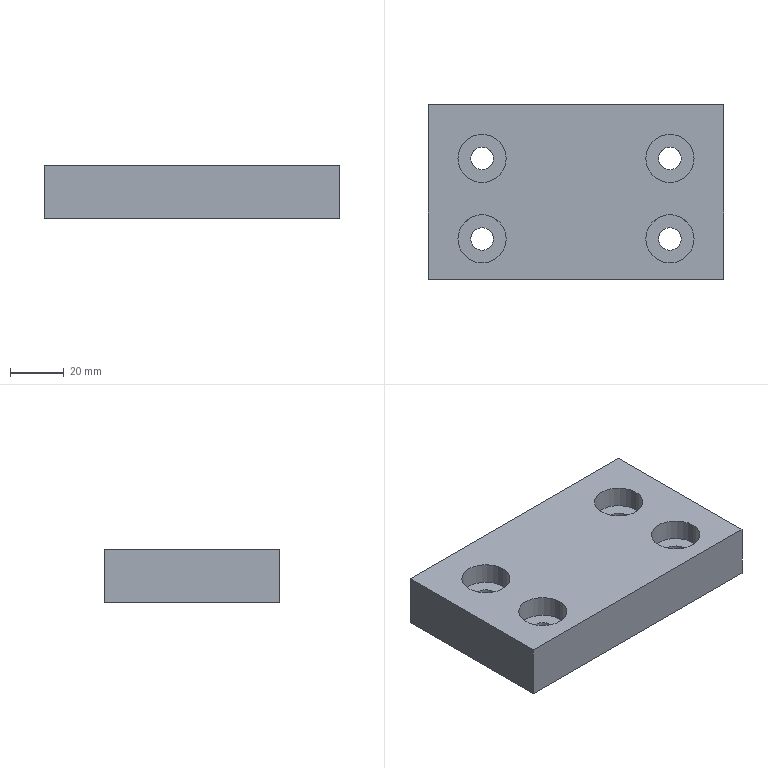Part | SolidWorks | features BaseBody 1 | 1 solid | 34 faces | box 110 x 65 x 20 mm | volume 129905 mm3 | cylinder 20 | plane 10 | cone 4 | commonest cylinder face diameters 8.4 x8 18 x8 10.2 x4
STEP:
#1=CARTESIAN_POINT('',(-264.2,110.,-32.879));
#2=VERTEX_POINT('',#1);
#3=CARTESIAN_POINT('',(-255.8,110.,-32.879));
#4=VERTEX_POINT('',#3);
#5=CARTESIAN_POINT('',(-260.,110.,-32.879));
#6=DIRECTION('',(0.,0.,1.));
#7=DIRECTION('',(1.,0.,0.));
#8=AXIS2_PLACEMENT_3D('',#5,#6,#7);
#9=CIRCLE('',#8,4.2);
#10=EDGE_CURVE('',#2,#4,#9,.T.);
#11=ORIENTED_EDGE('',*,*,#10,.F.);
#12=CARTESIAN_POINT('',(-264.2,110.,-20.879));
#13=VERTEX_POINT('',#12);
#14=CARTESIAN_POINT('',(-264.2,110.,-12.879));
#15=DIRECTION('',(0.,0.,1.));
#16=VECTOR('',#15,1000.);
#17=LINE('',#14,#16);
#18=EDGE_CURVE('',#2,#13,#17,.T.);
#19=ORIENTED_EDGE('',*,*,#18,.T.);
#20=CARTESIAN_POINT('',(-255.8,110.,-20.879));
#21=VERTEX_POINT('',#20);
#22=CARTESIAN_POINT('',(-260.,110.,-20.879));
#23=DIRECTION('',(0.,0.,-1.));
#24=DIRECTION('',(1.,0.,0.));
#25=AXIS2_PLACEMENT_3D('',#22,#23,#24);
#26=CIRCLE('',#25,4.2);
#27=EDGE_CURVE('',#21,#13,#26,.T.);
#28=ORIENTED_EDGE('',*,*,#27,.F.);
#29=CARTESIAN_POINT('',(-255.8,110.,-12.879));
#30=DIRECTION('',(0.,0.,1.));
#31=VECTOR('',#30,1000.);
#32=LINE('',#29,#31);
#33=EDGE_CURVE('',#4,#21,#32,.T.);
#34=ORIENTED_EDGE('',*,*,#33,.F.);
#35=EDGE_LOOP('',(#11,#19,#28,#34));
#36=FACE_OUTER_BOUND('',#35,.T.);
#37=CARTESIAN_POINT('',(-260.,110.,-12.879));
#38=DIRECTION('',(0.,0.,1.));
#39=DIRECTION('',(1.,0.,0.));
#40=AXIS2_PLACEMENT_3D('',#37,#38,#39);
#41=CYLINDRICAL_SURFACE('',#40,4.2);
#42=ADVANCED_FACE('',(#36),#41,.F.);
#43=CARTESIAN_POINT('',(-264.2,80.,-32.879));
#44=VERTEX_POINT('',#43);
#45=CARTESIAN_POINT('',(-255.8,80.,-32.879));
#46=VERTEX_POINT('',#45);
#47=CARTESIAN_POINT('',(-260.,80.,-32.879));
#48=DIRECTION('',(0.,0.,1.));
#49=DIRECTION('',(1.,0.,0.));
#50=AXIS2_PLACEMENT_3D('',#47,#48,#49);
#51=CIRCLE('',#50,4.2);
#52=EDGE_CURVE('',#44,#46,#51,.T.);
#53=ORIENTED_EDGE('',*,*,#52,.F.);
#54=CARTESIAN_POINT('',(-264.2,80.,-20.879));
#55=VERTEX_POINT('',#54);
#56=CARTESIAN_POINT('',(-264.2,80.,-12.879));
#57=DIRECTION('',(0.,0.,1.));
#58=VECTOR('',#57,1000.);
#59=LINE('',#56,#58);
#60=EDGE_CURVE('',#44,#55,#59,.T.);
#61=ORIENTED_EDGE('',*,*,#60,.T.);
#62=CARTESIAN_POINT('',(-255.8,80.,-20.879));
#63=VERTEX_POINT('',#62);
#64=CARTESIAN_POINT('',(-260.,80.,-20.879));
#65=DIRECTION('',(0.,0.,-1.));
#66=DIRECTION('',(1.,0.,0.));
#67=AXIS2_PLACEMENT_3D('',#64,#65,#66);
#68=CIRCLE('',#67,4.2);
#69=EDGE_CURVE('',#63,#55,#68,.T.);
#70=ORIENTED_EDGE('',*,*,#69,.F.);
#71=CARTESIAN_POINT('',(-255.8,80.,-12.879));
#72=DIRECTION('',(0.,0.,1.));
#73=VECTOR('',#72,1000.);
#74=LINE('',#71,#73);
#75=EDGE_CURVE('',#46,#63,#74,.T.);
#76=ORIENTED_EDGE('',*,*,#75,.F.);
#77=EDGE_LOOP('',(#53,#61,#70,#76));
#78=FACE_OUTER_BOUND('',#77,.T.);
#79=CARTESIAN_POINT('',(-260.,80.,-12.879));
#80=DIRECTION('',(0.,0.,1.));
#81=DIRECTION('',(1.,0.,0.));
#82=AXIS2_PLACEMENT_3D('',#79,#80,#81);
#83=CYLINDRICAL_SURFACE('',#82,4.2);
#84=ADVANCED_FACE('',(#78),#83,.F.);
#85=CARTESIAN_POINT('',(-194.2,80.,-32.879));
#86=VERTEX_POINT('',#85);
#87=CARTESIAN_POINT('',(-185.8,80.,-32.879));
#88=VERTEX_POINT('',#87);
#89=CARTESIAN_POINT('',(-190.,80.,-32.879));
#90=DIRECTION('',(0.,0.,1.));
#91=DIRECTION('',(1.,0.,0.));
#92=AXIS2_PLACEMENT_3D('',#89,#90,#91);
#93=CIRCLE('',#92,4.2);
#94=EDGE_CURVE('',#86,#88,#93,.T.);
#95=ORIENTED_EDGE('',*,*,#94,.F.);
#96=CARTESIAN_POINT('',(-194.2,80.,-20.879));
#97=VERTEX_POINT('',#96);
#98=CARTESIAN_POINT('',(-194.2,80.,-12.879));
#99=DIRECTION('',(0.,0.,1.));
#100=VECTOR('',#99,1000.);
#101=LINE('',#98,#100);
#102=EDGE_CURVE('',#86,#97,#101,.T.);
#103=ORIENTED_EDGE('',*,*,#102,.T.);
#104=CARTESIAN_POINT('',(-185.8,80.,-20.879));
#105=VERTEX_POINT('',#104);
#106=CARTESIAN_POINT('',(-190.,80.,-20.879));
#107=DIRECTION('',(0.,0.,-1.));
#108=DIRECTION('',(1.,0.,0.));
#109=AXIS2_PLACEMENT_3D('',#106,#107,#108);
#110=CIRCLE('',#109,4.2);
#111=EDGE_CURVE('',#105,#97,#110,.T.);
#112=ORIENTED_EDGE('',*,*,#111,.F.);
#113=CARTESIAN_POINT('',(-185.8,80.,-12.879));
#114=DIRECTION('',(0.,0.,1.));
#115=VECTOR('',#114,1000.);
#116=LINE('',#113,#115);
#117=EDGE_CURVE('',#88,#105,#116,.T.);
#118=ORIENTED_EDGE('',*,*,#117,.F.);
#119=EDGE_LOOP('',(#95,#103,#112,#118));
#120=FACE_OUTER_BOUND('',#119,.T.);
#121=CARTESIAN_POINT('',(-190.,80.,-12.879));
#122=DIRECTION('',(0.,0.,1.));
#123=DIRECTION('',(1.,0.,0.));
#124=AXIS2_PLACEMENT_3D('',#121,#122,#123);
#125=CYLINDRICAL_SURFACE('',#124,4.2);
#126=ADVANCED_FACE('',(#120),#125,.F.);
#127=CARTESIAN_POINT('',(-194.2,110.,-32.879));
#128=VERTEX_POINT('',#127);
#129=CARTESIAN_POINT('',(-185.8,110.,-32.879));
#130=VERTEX_POINT('',#129);
#131=CARTESIAN_POINT('',(-190.,110.,-32.879));
#132=DIRECTION('',(0.,0.,1.));
#133=DIRECTION('',(1.,0.,0.));
#134=AXIS2_PLACEMENT_3D('',#131,#132,#133);
#135=CIRCLE('',#134,4.2);
#136=EDGE_CURVE('',#128,#130,#135,.T.);
#137=ORIENTED_EDGE('',*,*,#136,.F.);
#138=CARTESIAN_POINT('',(-194.2,110.,-20.879));
#139=VERTEX_POINT('',#138);
#140=CARTESIAN_POINT('',(-194.2,110.,-12.879));
#141=DIRECTION('',(0.,0.,1.));
#142=VECTOR('',#141,1000.);
#143=LINE('',#140,#142);
#144=EDGE_CURVE('',#128,#139,#143,.T.);
#145=ORIENTED_EDGE('',*,*,#144,.T.);
#146=CARTESIAN_POINT('',(-185.8,110.,-20.879));
#147=VERTEX_POINT('',#146);
#148=CARTESIAN_POINT('',(-190.,110.,-20.879));
#149=DIRECTION('',(0.,0.,-1.));
#150=DIRECTION('',(1.,0.,0.));
#151=AXIS2_PLACEMENT_3D('',#148,#149,#150);
#152=CIRCLE('',#151,4.2);
#153=EDGE_CURVE('',#147,#139,#152,.T.);
#154=ORIENTED_EDGE('',*,*,#153,.F.);
#155=CARTESIAN_POINT('',(-185.8,110.,-12.879));
#156=DIRECTION('',(0.,0.,1.));
#157=VECTOR('',#156,1000.);
#158=LINE('',#155,#157);
#159=EDGE_CURVE('',#130,#147,#158,.T.);
#160=ORIENTED_EDGE('',*,*,#159,.F.);
#161=EDGE_LOOP('',(#137,#145,#154,#160));
#162=FACE_OUTER_BOUND('',#161,.T.);
#163=CARTESIAN_POINT('',(-190.,110.,-12.879));
#164=DIRECTION('',(0.,0.,1.));
#165=DIRECTION('',(1.,0.,0.));
#166=AXIS2_PLACEMENT_3D('',#163,#164,#165);
#167=CYLINDRICAL_SURFACE('',#166,4.2);
#168=ADVANCED_FACE('',(#162),#167,.F.);
#169=CARTESIAN_POINT('',(-178.,117.,-27.979));
#170=VERTEX_POINT('',#169);
#171=CARTESIAN_POINT('',(-178.,117.,-17.779));
#172=VERTEX_POINT('',#171);
#173=CARTESIAN_POINT('',(-178.,117.,-22.879));
#174=DIRECTION('',(0.,1.,0.));
#175=DIRECTION('',(0.,0.,1.));
#176=AXIS2_PLACEMENT_3D('',#173,#174,#175);
#177=CIRCLE('',#176,5.1);
#178=EDGE_CURVE('',#170,#172,#177,.T.);
#179=ORIENTED_EDGE('',*,*,#178,.F.);
#180=CARTESIAN_POINT('',(-178.,130.,-27.979));
#181=VERTEX_POINT('',#180);
#182=CARTESIAN_POINT('',(-178.,130.,-27.979));
#183=DIRECTION('',(0.,1.,0.));
#184=VECTOR('',#183,1000.);
#185=LINE('',#182,#184);
#186=EDGE_CURVE('',#170,#181,#185,.T.);
#187=ORIENTED_EDGE('',*,*,#186,.T.);
#188=CARTESIAN_POINT('',(-178.,130.,-17.779));
#189=VERTEX_POINT('',#188);
#190=CARTESIAN_POINT('',(-178.,130.,-22.879));
#191=DIRECTION('',(0.,1.,0.));
#192=DIRECTION('',(0.,0.,1.));
#193=AXIS2_PLACEMENT_3D('',#190,#191,#192);
#194=CIRCLE('',#193,5.1);
#195=EDGE_CURVE('',#181,#189,#194,.T.);
#196=ORIENTED_EDGE('',*,*,#195,.T.);
#197=CARTESIAN_POINT('',(-178.,130.,-17.779));
#198=DIRECTION('',(0.,1.,0.));
#199=VECTOR('',#198,1000.);
#200=LINE('',#197,#199);
#201=EDGE_CURVE('',#172,#189,#200,.T.);
#202=ORIENTED_EDGE('',*,*,#201,.F.);
#203=EDGE_LOOP('',(#179,#187,#196,#202));
#204=FACE_OUTER_BOUND('',#203,.T.);
#205=CARTESIAN_POINT('',(-178.,130.,-22.879));
#206=DIRECTION('',(0.,1.,0.));
#207=DIRECTION('',(0.,0.,1.));
#208=AXIS2_PLACEMENT_3D('',#205,#206,#207);
#209=CYLINDRICAL_SURFACE('',#208,5.1);
#210=ADVANCED_FACE('',(#204),#209,.F.);
#211=CARTESIAN_POINT('',(-272.,117.,-27.979));
#212=VERTEX_POINT('',#211);
#213=CARTESIAN_POINT('',(-272.,117.,-17.779));
#214=VERTEX_POINT('',#213);
#215=CARTESIAN_POINT('',(-272.,117.,-22.879));
#216=DIRECTION('',(0.,1.,0.));
#217=DIRECTION('',(0.,0.,1.));
#218=AXIS2_PLACEMENT_3D('',#215,#216,#217);
#219=CIRCLE('',#218,5.1);
#220=EDGE_CURVE('',#212,#214,#219,.T.);
#221=ORIENTED_EDGE('',*,*,#220,.F.);
#222=CARTESIAN_POINT('',(-272.,130.,-27.979));
#223=VERTEX_POINT('',#222);
#224=CARTESIAN_POINT('',(-272.,130.,-27.979));
#225=DIRECTION('',(0.,1.,0.));
#226=VECTOR('',#225,1000.);
#227=LINE('',#224,#226);
#228=EDGE_CURVE('',#212,#223,#227,.T.);
#229=ORIENTED_EDGE('',*,*,#228,.T.);
#230=CARTESIAN_POINT('',(-272.,130.,-17.779));
#231=VERTEX_POINT('',#230);
#232=CARTESIAN_POINT('',(-272.,130.,-22.879));
#233=DIRECTION('',(0.,1.,0.));
#234=DIRECTION('',(0.,0.,1.));
#235=AXIS2_PLACEMENT_3D('',#232,#233,#234);
#236=CIRCLE('',#235,5.1);
#237=EDGE_CURVE('',#223,#231,#236,.T.);
#238=ORIENTED_EDGE('',*,*,#237,.T.);
#239=CARTESIAN_POINT('',(-272.,130.,-17.779));
#240=DIRECTION('',(0.,1.,0.));
#241=VECTOR('',#240,1000.);
#242=LINE('',#239,#241);
#243=EDGE_CURVE('',#214,#231,#242,.T.);
#244=ORIENTED_EDGE('',*,*,#243,.F.);
#245=EDGE_LOOP('',(#221,#229,#238,#244));
#246=FACE_OUTER_BOUND('',#245,.T.);
#247=CARTESIAN_POINT('',(-272.,130.,-22.879));
#248=DIRECTION('',(0.,1.,0.));
#249=DIRECTION('',(0.,0.,1.));
#250=AXIS2_PLACEMENT_3D('',#247,#248,#249);
#251=CYLINDRICAL_SURFACE('',#250,5.1);
#252=ADVANCED_FACE('',(#246),#251,.F.);
#253=CARTESIAN_POINT('',(-251.,110.,-20.879));
#254=VERTEX_POINT('',#253);
#255=CARTESIAN_POINT('',(-269.,110.,-20.879));
#256=VERTEX_POINT('',#255);
#257=CARTESIAN_POINT('',(-260.,110.,-20.879));
#258=DIRECTION('',(0.,0.,-1.));
#259=DIRECTION('',(1.,0.,0.));
#260=AXIS2_PLACEMENT_3D('',#257,#258,#259);
#261=CIRCLE('',#260,9.);
#262=EDGE_CURVE('',#254,#256,#261,.T.);
#263=ORIENTED_EDGE('',*,*,#262,.T.);
#264=CARTESIAN_POINT('',(-269.,110.,-12.879));
#265=VERTEX_POINT('',#264);
#266=CARTESIAN_POINT('',(-269.,110.,-12.879));
#267=DIRECTION('',(0.,0.,1.));
#268=VECTOR('',#267,1000.);
#269=LINE('',#266,#268);
#270=EDGE_CURVE('',#256,#265,#269,.T.);
#271=ORIENTED_EDGE('',*,*,#270,.T.);
#272=CARTESIAN_POINT('',(-251.,110.,-12.879));
#273=VERTEX_POINT('',#272);
#274=CARTESIAN_POINT('',(-260.,110.,-12.879));
#275=DIRECTION('',(0.,0.,1.));
#276=DIRECTION('',(1.,0.,0.));
#277=AXIS2_PLACEMENT_3D('',#274,#275,#276);
#278=CIRCLE('',#277,9.);
#279=EDGE_CURVE('',#265,#273,#278,.T.);
#280=ORIENTED_EDGE('',*,*,#279,.T.);
#281=CARTESIAN_POINT('',(-251.,110.,-12.879));
#282=DIRECTION('',(0.,0.,1.));
#283=VECTOR('',#282,1000.);
#284=LINE('',#281,#283);
#285=EDGE_CURVE('',#254,#273,#284,.T.);
#286=ORIENTED_EDGE('',*,*,#285,.F.);
#287=EDGE_LOOP('',(#263,#271,#280,#286));
#288=FACE_OUTER_BOUND('',#287,.T.);
#289=CARTESIAN_POINT('',(-260.,110.,-12.879));
#290=DIRECTION('',(0.,0.,1.));
#291=DIRECTION('',(1.,0.,0.));
#292=AXIS2_PLACEMENT_3D('',#289,#290,#291);
#293=CYLINDRICAL_SURFACE('',#292,9.);
#294=ADVANCED_FACE('',(#288),#293,.F.);
#295=CARTESIAN_POINT('',(-251.,80.,-20.879));
#296=VERTEX_POINT('',#295);
#297=CARTESIAN_POINT('',(-269.,80.,-20.879));
#298=VERTEX_POINT('',#297);
#299=CARTESIAN_POINT('',(-260.,80.,-20.879));
#300=DIRECTION('',(0.,0.,-1.));
#301=DIRECTION('',(1.,0.,0.));
#302=AXIS2_PLACEMENT_3D('',#299,#300,#301);
#303=CIRCLE('',#302,9.);
#304=EDGE_CURVE('',#296,#298,#303,.T.);
#305=ORIENTED_EDGE('',*,*,#304,.T.);
#306=CARTESIAN_POINT('',(-269.,80.,-12.879));
#307=VERTEX_POINT('',#306);
#308=CARTESIAN_POINT('',(-269.,80.,-12.879));
#309=DIRECTION('',(0.,0.,1.));
#310=VECTOR('',#309,1000.);
#311=LINE('',#308,#310);
#312=EDGE_CURVE('',#298,#307,#311,.T.);
#313=ORIENTED_EDGE('',*,*,#312,.T.);
#314=CARTESIAN_POINT('',(-251.,80.,-12.879));
#315=VERTEX_POINT('',#314);
#316=CARTESIAN_POINT('',(-260.,80.,-12.879));
#317=DIRECTION('',(0.,0.,1.));
#318=DIRECTION('',(1.,0.,0.));
#319=AXIS2_PLACEMENT_3D('',#316,#317,#318);
#320=CIRCLE('',#319,9.);
#321=EDGE_CURVE('',#307,#315,#320,.T.);
#322=ORIENTED_EDGE('',*,*,#321,.T.);
#323=CARTESIAN_POINT('',(-251.,80.,-12.879));
#324=DIRECTION('',(0.,0.,1.));
#325=VECTOR('',#324,1000.);
#326=LINE('',#323,#325);
#327=EDGE_CURVE('',#296,#315,#326,.T.);
#328=ORIENTED_EDGE('',*,*,#327,.F.);
#329=EDGE_LOOP('',(#305,#313,#322,#328));
#330=FACE_OUTER_BOUND('',#329,.T.);
#331=CARTESIAN_POINT('',(-260.,80.,-12.879));
#332=DIRECTION('',(0.,0.,1.));
#333=DIRECTION('',(1.,0.,0.));
#334=AXIS2_PLACEMENT_3D('',#331,#332,#333);
#335=CYLINDRICAL_SURFACE('',#334,9.);
#336=ADVANCED_FACE('',(#330),#335,.F.);
#337=CARTESIAN_POINT('',(-181.,80.,-20.879));
#338=VERTEX_POINT('',#337);
#339=CARTESIAN_POINT('',(-199.,80.,-20.879));
#340=VERTEX_POINT('',#339);
#341=CARTESIAN_POINT('',(-190.,80.,-20.879));
#342=DIRECTION('',(0.,0.,-1.));
#343=DIRECTION('',(1.,0.,0.));
#344=AXIS2_PLACEMENT_3D('',#341,#342,#343);
#345=CIRCLE('',#344,9.);
#346=EDGE_CURVE('',#338,#340,#345,.T.);
#347=ORIENTED_EDGE('',*,*,#346,.T.);
#348=CARTESIAN_POINT('',(-199.,80.,-12.879));
#349=VERTEX_POINT('',#348);
#350=CARTESIAN_POINT('',(-199.,80.,-12.879));
#351=DIRECTION('',(0.,0.,1.));
#352=VECTOR('',#351,1000.);
#353=LINE('',#350,#352);
#354=EDGE_CURVE('',#340,#349,#353,.T.);
#355=ORIENTED_EDGE('',*,*,#354,.T.);
#356=CARTESIAN_POINT('',(-181.,80.,-12.879));
#357=VERTEX_POINT('',#356);
#358=CARTESIAN_POINT('',(-190.,80.,-12.879));
#359=DIRECTION('',(0.,0.,1.));
#360=DIRECTION('',(1.,0.,0.));
#361=AXIS2_PLACEMENT_3D('',#358,#359,#360);
#362=CIRCLE('',#361,9.);
#363=EDGE_CURVE('',#349,#357,#362,.T.);
#364=ORIENTED_EDGE('',*,*,#363,.T.);
#365=CARTESIAN_POINT('',(-181.,80.,-12.879));
#366=DIRECTION('',(0.,0.,1.));
#367=VECTOR('',#366,1000.);
#368=LINE('',#365,#367);
#369=EDGE_CURVE('',#338,#357,#368,.T.);
#370=ORIENTED_EDGE('',*,*,#369,.F.);
#371=EDGE_LOOP('',(#347,#355,#364,#370));
#372=FACE_OUTER_BOUND('',#371,.T.);
#373=CARTESIAN_POINT('',(-190.,80.,-12.879));
#374=DIRECTION('',(0.,0.,1.));
#375=DIRECTION('',(1.,0.,0.));
#376=AXIS2_PLACEMENT_3D('',#373,#374,#375);
#377=CYLINDRICAL_SURFACE('',#376,9.);
#378=ADVANCED_FACE('',(#372),#377,.F.);
#379=CARTESIAN_POINT('',(-181.,110.,-20.879));
#380=VERTEX_POINT('',#379);
#381=CARTESIAN_POINT('',(-199.,110.,-20.879));
#382=VERTEX_POINT('',#381);
#383=CARTESIAN_POINT('',(-190.,110.,-20.879));
#384=DIRECTION('',(0.,0.,-1.));
#385=DIRECTION('',(1.,0.,0.));
#386=AXIS2_PLACEMENT_3D('',#383,#384,#385);
#387=CIRCLE('',#386,9.);
#388=EDGE_CURVE('',#380,#382,#387,.T.);
#389=ORIENTED_EDGE('',*,*,#388,.T.);
#390=CARTESIAN_POINT('',(-199.,110.,-12.879));
#391=VERTEX_POINT('',#390);
#392=CARTESIAN_POINT('',(-199.,110.,-12.879));
#393=DIRECTION('',(0.,0.,1.));
#394=VECTOR('',#393,1000.);
#395=LINE('',#392,#394);
#396=EDGE_CURVE('',#382,#391,#395,.T.);
#397=ORIENTED_EDGE('',*,*,#396,.T.);
#398=CARTESIAN_POINT('',(-181.,110.,-12.879));
#399=VERTEX_POINT('',#398);
#400=CARTESIAN_POINT('',(-190.,110.,-12.879));
#401=DIRECTION('',(0.,0.,1.));
#402=DIRECTION('',(1.,0.,0.));
#403=AXIS2_PLACEMENT_3D('',#400,#401,#402);
#404=CIRCLE('',#403,9.);
#405=EDGE_CURVE('',#391,#399,#404,.T.);
#406=ORIENTED_EDGE('',*,*,#405,.T.);
#407=CARTESIAN_POINT('',(-181.,110.,-12.879));
#408=DIRECTION('',(0.,0.,1.));
#409=VECTOR('',#408,1000.);
#410=LINE('',#407,#409);
#411=EDGE_CURVE('',#380,#399,#410,.T.);
#412=ORIENTED_EDGE('',*,*,#411,.F.);
#413=EDGE_LOOP('',(#389,#397,#406,#412));
#414=FACE_OUTER_BOUND('',#413,.T.);
#415=CARTESIAN_POINT('',(-190.,110.,-12.879));
#416=DIRECTION('',(0.,0.,1.));
#417=DIRECTION('',(1.,0.,0.));
#418=AXIS2_PLACEMENT_3D('',#415,#416,#417);
#419=CYLINDRICAL_SURFACE('',#418,9.);
#420=ADVANCED_FACE('',(#414),#419,.F.);
#421=CARTESIAN_POINT('',(-178.,113.936,-22.879));
#422=VERTEX_POINT('',#421);
#423=CARTESIAN_POINT('',(-178.,117.,-17.779));
#424=DIRECTION('',(0.,0.515,0.8572));
#425=VECTOR('',#424,1000.);
#426=LINE('',#423,#425);
#427=EDGE_CURVE('',#422,#172,#426,.T.);
#428=ORIENTED_EDGE('',*,*,#427,.F.);
#429=CARTESIAN_POINT('',(-178.,117.,-27.979));
#430=DIRECTION('',(0.,0.515,-0.8572));
#431=VECTOR('',#430,1000.);
#432=LINE('',#429,#431);
#433=EDGE_CURVE('',#422,#170,#432,.T.);
#434=ORIENTED_EDGE('',*,*,#433,.T.);
#435=ORIENTED_EDGE('',*,*,#178,.T.);
#436=EDGE_LOOP('',(#428,#434,#435));
#437=FACE_OUTER_BOUND('',#436,.T.);
#438=CARTESIAN_POINT('',(-178.,117.,-22.879));
#439=DIRECTION('',(0.,1.,0.));
#440=DIRECTION('',(0.,0.,1.));
#441=AXIS2_PLACEMENT_3D('',#438,#439,#440);
#442=CONICAL_SURFACE('',#441,5.1,1.03);
#443=ADVANCED_FACE('',(#437),#442,.F.);
#444=CARTESIAN_POINT('',(-272.,113.936,-22.879));
#445=VERTEX_POINT('',#444);
#446=CARTESIAN_POINT('',(-272.,117.,-17.779));
#447=DIRECTION('',(0.,0.515,0.8572));
#448=VECTOR('',#447,1000.);
#449=LINE('',#446,#448);
#450=EDGE_CURVE('',#445,#214,#449,.T.);
#451=ORIENTED_EDGE('',*,*,#450,.F.);
#452=CARTESIAN_POINT('',(-272.,117.,-27.979));
#453=DIRECTION('',(0.,0.515,-0.8572));
#454=VECTOR('',#453,1000.);
#455=LINE('',#452,#454);
#456=EDGE_CURVE('',#445,#212,#455,.T.);
#457=ORIENTED_EDGE('',*,*,#456,.T.);
#458=ORIENTED_EDGE('',*,*,#220,.T.);
#459=EDGE_LOOP('',(#451,#457,#458));
#460=FACE_OUTER_BOUND('',#459,.T.);
#461=CARTESIAN_POINT('',(-272.,117.,-22.879));
#462=DIRECTION('',(0.,1.,0.));
#463=DIRECTION('',(0.,0.,1.));
#464=AXIS2_PLACEMENT_3D('',#461,#462,#463);
#465=CONICAL_SURFACE('',#464,5.1,1.03);
#466=ADVANCED_FACE('',(#460),#465,.F.);
#467=CARTESIAN_POINT('',(-280.,65.,-32.879));
#468=VERTEX_POINT('',#467);
#469=CARTESIAN_POINT('',(-280.,130.,-32.879));
#470=VERTEX_POINT('',#469);
#471=CARTESIAN_POINT('',(-280.,100.,-32.879));
#472=DIRECTION('',(0.,1.,0.));
#473=VECTOR('',#472,1000.);
#474=LINE('',#471,#473);
#475=EDGE_CURVE('',#468,#470,#474,.T.);
#476=ORIENTED_EDGE('',*,*,#475,.T.);
#477=CARTESIAN_POINT('',(-170.,130.,-32.879));
#478=VERTEX_POINT('',#477);
#479=CARTESIAN_POINT('',(-225.,130.,-32.879));
#480=DIRECTION('',(1.,0.,0.));
#481=VECTOR('',#480,1000.);
#482=LINE('',#479,#481);
#483=EDGE_CURVE('',#470,#478,#482,.T.);
#484=ORIENTED_EDGE('',*,*,#483,.T.);
#485=CARTESIAN_POINT('',(-170.,65.,-32.879));
#486=VERTEX_POINT('',#485);
#487=CARTESIAN_POINT('',(-170.,100.,-32.879));
#488=DIRECTION('',(0.,-1.,0.));
#489=VECTOR('',#488,1000.);
#490=LINE('',#487,#489);
#491=EDGE_CURVE('',#478,#486,#490,.T.);
#492=ORIENTED_EDGE('',*,*,#491,.T.);
#493=CARTESIAN_POINT('',(-225.,65.,-32.879));
#494=DIRECTION('',(-1.,0.,0.));
#495=VECTOR('',#494,1000.);
#496=LINE('',#493,#495);
#497=EDGE_CURVE('',#486,#468,#496,.T.);
#498=ORIENTED_EDGE('',*,*,#497,.T.);
#499=EDGE_LOOP('',(#476,#484,#492,#498));
#500=FACE_OUTER_BOUND('',#499,.T.);
#501=CARTESIAN_POINT('',(-260.,110.,-32.879));
#502=DIRECTION('',(0.,0.,1.));
#503=DIRECTION('',(1.,0.,0.));
#504=AXIS2_PLACEMENT_3D('',#501,#502,#503);
#505=CIRCLE('',#504,4.2);
#506=EDGE_CURVE('',#4,#2,#505,.T.);
#507=ORIENTED_EDGE('',*,*,#506,.T.);
#508=ORIENTED_EDGE('',*,*,#10,.T.);
#509=EDGE_LOOP('',(#507,#508));
#510=FACE_BOUND('',#509,.T.);
#511=CARTESIAN_POINT('',(-260.,80.,-32.879));
#512=DIRECTION('',(0.,0.,1.));
#513=DIRECTION('',(1.,0.,0.));
#514=AXIS2_PLACEMENT_3D('',#511,#512,#513);
#515=CIRCLE('',#514,4.2);
#516=EDGE_CURVE('',#46,#44,#515,.T.);
#517=ORIENTED_EDGE('',*,*,#516,.T.);
#518=ORIENTED_EDGE('',*,*,#52,.T.);
#519=EDGE_LOOP('',(#517,#518));
#520=FACE_BOUND('',#519,.T.);
#521=CARTESIAN_POINT('',(-190.,80.,-32.879));
#522=DIRECTION('',(0.,0.,1.));
#523=DIRECTION('',(1.,0.,0.));
#524=AXIS2_PLACEMENT_3D('',#521,#522,#523);
#525=CIRCLE('',#524,4.2);
#526=EDGE_CURVE('',#88,#86,#525,.T.);
#527=ORIENTED_EDGE('',*,*,#526,.T.);
#528=ORIENTED_EDGE('',*,*,#94,.T.);
#529=EDGE_LOOP('',(#527,#528));
#530=FACE_BOUND('',#529,.T.);
#531=CARTESIAN_POINT('',(-190.,110.,-32.879));
#532=DIRECTION('',(0.,0.,1.));
#533=DIRECTION('',(1.,0.,0.));
#534=AXIS2_PLACEMENT_3D('',#531,#532,#533);
#535=CIRCLE('',#534,4.2);
#536=EDGE_CURVE('',#130,#128,#535,.T.);
#537=ORIENTED_EDGE('',*,*,#536,.T.);
#538=ORIENTED_EDGE('',*,*,#136,.T.);
#539=EDGE_LOOP('',(#537,#538));
#540=FACE_BOUND('',#539,.T.);
#541=CARTESIAN_POINT('',(-225.,100.,-32.879));
#542=DIRECTION('',(0.,0.,-1.));
#543=DIRECTION('',(-1.,0.,0.));
#544=AXIS2_PLACEMENT_3D('',#541,#542,#543);
#545=PLANE('',#544);
#546=ADVANCED_FACE('',(#500,#510,#520,#530,#540),#545,.T.);
#547=CARTESIAN_POINT('',(-280.,130.,-12.879));
#548=VERTEX_POINT('',#547);
#549=CARTESIAN_POINT('',(-280.,130.,-12.879));
#550=DIRECTION('',(0.,0.,-1.));
#551=VECTOR('',#550,1000.);
#552=LINE('',#549,#551);
#553=EDGE_CURVE('',#548,#470,#552,.T.);
#554=ORIENTED_EDGE('',*,*,#553,.F.);
#555=CARTESIAN_POINT('',(-170.,130.,-12.879));
#556=VERTEX_POINT('',#555);
#557=CARTESIAN_POINT('',(-280.,130.,-12.879));
#558=DIRECTION('',(-1.,0.,0.));
#559=VECTOR('',#558,1000.);
#560=LINE('',#557,#559);
#561=EDGE_CURVE('',#556,#548,#560,.T.);
#562=ORIENTED_EDGE('',*,*,#561,.F.);
#563=CARTESIAN_POINT('',(-170.,130.,-12.879));
#564=DIRECTION('',(0.,0.,1.));
#565=VECTOR('',#564,1000.);
#566=LINE('',#563,#565);
#567=EDGE_CURVE('',#478,#556,#566,.T.);
#568=ORIENTED_EDGE('',*,*,#567,.F.);
#569=ORIENTED_EDGE('',*,*,#483,.F.);
#570=EDGE_LOOP('',(#554,#562,#568,#569));
#571=FACE_OUTER_BOUND('',#570,.T.);
#572=CARTESIAN_POINT('',(-178.,130.,-22.879));
#573=DIRECTION('',(0.,1.,0.));
#574=DIRECTION('',(0.,0.,1.));
#575=AXIS2_PLACEMENT_3D('',#572,#573,#574);
#576=CIRCLE('',#575,5.1);
#577=EDGE_CURVE('',#189,#181,#576,.T.);
#578=ORIENTED_EDGE('',*,*,#577,.F.);
#579=ORIENTED_EDGE('',*,*,#195,.F.);
#580=EDGE_LOOP('',(#578,#579));
#581=FACE_BOUND('',#580,.T.);
#582=CARTESIAN_POINT('',(-272.,130.,-22.879));
#583=DIRECTION('',(0.,1.,0.));
#584=DIRECTION('',(0.,0.,1.));
#585=AXIS2_PLACEMENT_3D('',#582,#583,#584);
#586=CIRCLE('',#585,5.1);
#587=EDGE_CURVE('',#231,#223,#586,.T.);
#588=ORIENTED_EDGE('',*,*,#587,.F.);
#589=ORIENTED_EDGE('',*,*,#237,.F.);
#590=EDGE_LOOP('',(#588,#589));
#591=FACE_BOUND('',#590,.T.);
#592=CARTESIAN_POINT('',(-280.,130.,-12.879));
#593=DIRECTION('',(0.,-1.,0.));
#594=DIRECTION('',(0.,0.,-1.));
#595=AXIS2_PLACEMENT_3D('',#592,#593,#594);
#596=PLANE('',#595);
#597=ADVANCED_FACE('',(#571,#581,#591),#596,.F.);
#598=CARTESIAN_POINT('',(-280.,65.,-12.879));
#599=VERTEX_POINT('',#598);
#600=CARTESIAN_POINT('',(-280.,65.,-12.879));
#601=DIRECTION('',(0.,0.,-1.));
#602=VECTOR('',#601,1000.);
#603=LINE('',#600,#602);
#604=EDGE_CURVE('',#599,#468,#603,.T.);
#605=ORIENTED_EDGE('',*,*,#604,.F.);
#606=CARTESIAN_POINT('',(-280.,70.,-12.879));
#607=DIRECTION('',(0.,-1.,0.));
#608=VECTOR('',#607,1000.);
#609=LINE('',#606,#608);
#610=EDGE_CURVE('',#548,#599,#609,.T.);
#611=ORIENTED_EDGE('',*,*,#610,.F.);
#612=ORIENTED_EDGE('',*,*,#553,.T.);
#613=ORIENTED_EDGE('',*,*,#475,.F.);
#614=EDGE_LOOP('',(#605,#611,#612,#613));
#615=FACE_OUTER_BOUND('',#614,.T.);
#616=CARTESIAN_POINT('',(-280.,70.,-12.879));
#617=DIRECTION('',(1.,0.,0.));
#618=DIRECTION('',(0.,0.,-1.));
#619=AXIS2_PLACEMENT_3D('',#616,#617,#618);
#620=PLANE('',#619);
#621=ADVANCED_FACE('',(#615),#620,.F.);
#622=CARTESIAN_POINT('',(-170.,65.,-12.879));
#623=VERTEX_POINT('',#622);
#624=CARTESIAN_POINT('',(-170.,65.,-12.879));
#625=DIRECTION('',(0.,0.,-1.));
#626=VECTOR('',#625,1000.);
#627=LINE('',#624,#626);
#628=EDGE_CURVE('',#623,#486,#627,.T.);
#629=ORIENTED_EDGE('',*,*,#628,.F.);
#630=CARTESIAN_POINT('',(-280.,65.,-12.879));
#631=DIRECTION('',(1.,0.,0.));
#632=VECTOR('',#631,1000.);
#633=LINE('',#630,#632);
#634=EDGE_CURVE('',#599,#623,#633,.T.);
#635=ORIENTED_EDGE('',*,*,#634,.F.);
#636=ORIENTED_EDGE('',*,*,#604,.T.);
#637=ORIENTED_EDGE('',*,*,#497,.F.);
#638=EDGE_LOOP('',(#629,#635,#636,#637));
#639=FACE_OUTER_BOUND('',#638,.T.);
#640=CARTESIAN_POINT('',(-280.,65.,-12.879));
#641=DIRECTION('',(0.,1.,0.));
#642=DIRECTION('',(0.,0.,1.));
#643=AXIS2_PLACEMENT_3D('',#640,#641,#642);
#644=PLANE('',#643);
#645=ADVANCED_FACE('',(#639),#644,.F.);
#646=ORIENTED_EDGE('',*,*,#567,.T.);
#647=CARTESIAN_POINT('',(-170.,70.,-12.879));
#648=DIRECTION('',(0.,1.,0.));
#649=VECTOR('',#648,1000.);
#650=LINE('',#647,#649);
#651=EDGE_CURVE('',#623,#556,#650,.T.);
#652=ORIENTED_EDGE('',*,*,#651,.F.);
#653=ORIENTED_EDGE('',*,*,#628,.T.);
#654=ORIENTED_EDGE('',*,*,#491,.F.);
#655=EDGE_LOOP('',(#646,#652,#653,#654));
#656=FACE_OUTER_BOUND('',#655,.T.);
#657=CARTESIAN_POINT('',(-170.,70.,-12.879));
#658=DIRECTION('',(-1.,0.,0.));
#659=DIRECTION('',(0.,0.,1.));
#660=AXIS2_PLACEMENT_3D('',#657,#658,#659);
#661=PLANE('',#660);
#662=ADVANCED_FACE('',(#656),#661,.F.);
#663=ORIENTED_EDGE('',*,*,#18,.F.);
#664=ORIENTED_EDGE('',*,*,#506,.F.);
#665=ORIENTED_EDGE('',*,*,#33,.T.);
#666=CARTESIAN_POINT('',(-260.,110.,-20.879));
#667=DIRECTION('',(0.,0.,-1.));
#668=DIRECTION('',(1.,0.,0.));
#669=AXIS2_PLACEMENT_3D('',#666,#667,#668);
#670=CIRCLE('',#669,4.2);
#671=EDGE_CURVE('',#13,#21,#670,.T.);
#672=ORIENTED_EDGE('',*,*,#671,.F.);
#673=EDGE_LOOP('',(#663,#664,#665,#672));
#674=FACE_OUTER_BOUND('',#673,.T.);
#675=CARTESIAN_POINT('',(-260.,110.,-12.879));
#676=DIRECTION('',(0.,0.,1.));
#677=DIRECTION('',(1.,0.,0.));
#678=AXIS2_PLACEMENT_3D('',#675,#676,#677);
#679=CYLINDRICAL_SURFACE('',#678,4.2);
#680=ADVANCED_FACE('',(#674),#679,.F.);
#681=ORIENTED_EDGE('',*,*,#60,.F.);
#682=ORIENTED_EDGE('',*,*,#516,.F.);
#683=ORIENTED_EDGE('',*,*,#75,.T.);
#684=CARTESIAN_POINT('',(-260.,80.,-20.879));
#685=DIRECTION('',(0.,0.,-1.));
#686=DIRECTION('',(1.,0.,0.));
#687=AXIS2_PLACEMENT_3D('',#684,#685,#686);
#688=CIRCLE('',#687,4.2);
#689=EDGE_CURVE('',#55,#63,#688,.T.);
#690=ORIENTED_EDGE('',*,*,#689,.F.);
#691=EDGE_LOOP('',(#681,#682,#683,#690));
#692=FACE_OUTER_BOUND('',#691,.T.);
#693=CARTESIAN_POINT('',(-260.,80.,-12.879));
#694=DIRECTION('',(0.,0.,1.));
#695=DIRECTION('',(1.,0.,0.));
#696=AXIS2_PLACEMENT_3D('',#693,#694,#695);
#697=CYLINDRICAL_SURFACE('',#696,4.2);
#698=ADVANCED_FACE('',(#692),#697,.F.);
#699=ORIENTED_EDGE('',*,*,#102,.F.);
#700=ORIENTED_EDGE('',*,*,#526,.F.);
#701=ORIENTED_EDGE('',*,*,#117,.T.);
#702=CARTESIAN_POINT('',(-190.,80.,-20.879));
#703=DIRECTION('',(0.,0.,-1.));
#704=DIRECTION('',(1.,0.,0.));
#705=AXIS2_PLACEMENT_3D('',#702,#703,#704);
#706=CIRCLE('',#705,4.2);
#707=EDGE_CURVE('',#97,#105,#706,.T.);
#708=ORIENTED_EDGE('',*,*,#707,.F.);
#709=EDGE_LOOP('',(#699,#700,#701,#708));
#710=FACE_OUTER_BOUND('',#709,.T.);
#711=CARTESIAN_POINT('',(-190.,80.,-12.879));
#712=DIRECTION('',(0.,0.,1.));
#713=DIRECTION('',(1.,0.,0.));
#714=AXIS2_PLACEMENT_3D('',#711,#712,#713);
#715=CYLINDRICAL_SURFACE('',#714,4.2);
#716=ADVANCED_FACE('',(#710),#715,.F.);
#717=ORIENTED_EDGE('',*,*,#144,.F.);
#718=ORIENTED_EDGE('',*,*,#536,.F.);
#719=ORIENTED_EDGE('',*,*,#159,.T.);
#720=CARTESIAN_POINT('',(-190.,110.,-20.879));
#721=DIRECTION('',(0.,0.,-1.));
#722=DIRECTION('',(1.,0.,0.));
#723=AXIS2_PLACEMENT_3D('',#720,#721,#722);
#724=CIRCLE('',#723,4.2);
#725=EDGE_CURVE('',#139,#147,#724,.T.);
#726=ORIENTED_EDGE('',*,*,#725,.F.);
#727=EDGE_LOOP('',(#717,#718,#719,#726));
#728=FACE_OUTER_BOUND('',#727,.T.);
#729=CARTESIAN_POINT('',(-190.,110.,-12.879));
#730=DIRECTION('',(0.,0.,1.));
#731=DIRECTION('',(1.,0.,0.));
#732=AXIS2_PLACEMENT_3D('',#729,#730,#731);
#733=CYLINDRICAL_SURFACE('',#732,4.2);
#734=ADVANCED_FACE('',(#728),#733,.F.);
#735=ORIENTED_EDGE('',*,*,#561,.T.);
#736=ORIENTED_EDGE('',*,*,#610,.T.);
#737=ORIENTED_EDGE('',*,*,#634,.T.);
#738=ORIENTED_EDGE('',*,*,#651,.T.);
#739=EDGE_LOOP('',(#735,#736,#737,#738));
#740=FACE_OUTER_BOUND('',#739,.T.);
#741=CARTESIAN_POINT('',(-260.,110.,-12.879));
#742=DIRECTION('',(0.,0.,1.));
#743=DIRECTION('',(1.,0.,0.));
#744=AXIS2_PLACEMENT_3D('',#741,#742,#743);
#745=CIRCLE('',#744,9.);
#746=EDGE_CURVE('',#273,#265,#745,.T.);
#747=ORIENTED_EDGE('',*,*,#746,.F.);
#748=ORIENTED_EDGE('',*,*,#279,.F.);
#749=EDGE_LOOP('',(#747,#748));
#750=FACE_BOUND('',#749,.T.);
#751=CARTESIAN_POINT('',(-260.,80.,-12.879));
#752=DIRECTION('',(0.,0.,1.));
#753=DIRECTION('',(1.,0.,0.));
#754=AXIS2_PLACEMENT_3D('',#751,#752,#753);
#755=CIRCLE('',#754,9.);
#756=EDGE_CURVE('',#315,#307,#755,.T.);
#757=ORIENTED_EDGE('',*,*,#756,.F.);
#758=ORIENTED_EDGE('',*,*,#321,.F.);
#759=EDGE_LOOP('',(#757,#758));
#760=FACE_BOUND('',#759,.T.);
#761=CARTESIAN_POINT('',(-190.,80.,-12.879));
#762=DIRECTION('',(0.,0.,1.));
#763=DIRECTION('',(1.,0.,0.));
#764=AXIS2_PLACEMENT_3D('',#761,#762,#763);
#765=CIRCLE('',#764,9.);
#766=EDGE_CURVE('',#357,#349,#765,.T.);
#767=ORIENTED_EDGE('',*,*,#766,.F.);
#768=ORIENTED_EDGE('',*,*,#363,.F.);
#769=EDGE_LOOP('',(#767,#768));
#770=FACE_BOUND('',#769,.T.);
#771=CARTESIAN_POINT('',(-190.,110.,-12.879));
#772=DIRECTION('',(0.,0.,1.));
#773=DIRECTION('',(1.,0.,0.));
#774=AXIS2_PLACEMENT_3D('',#771,#772,#773);
#775=CIRCLE('',#774,9.);
#776=EDGE_CURVE('',#399,#391,#775,.T.);
#777=ORIENTED_EDGE('',*,*,#776,.F.);
#778=ORIENTED_EDGE('',*,*,#405,.F.);
#779=EDGE_LOOP('',(#777,#778));
#780=FACE_BOUND('',#779,.T.);
#781=CARTESIAN_POINT('',(-225.,100.,-12.879));
#782=DIRECTION('',(0.,0.,-1.));
#783=DIRECTION('',(-1.,0.,0.));
#784=AXIS2_PLACEMENT_3D('',#781,#782,#783);
#785=PLANE('',#784);
#786=ADVANCED_FACE('',(#740,#750,#760,#770,#780),#785,.F.);
#787=ORIENTED_EDGE('',*,*,#186,.F.);
#788=CARTESIAN_POINT('',(-178.,117.,-22.879));
#789=DIRECTION('',(0.,1.,0.));
#790=DIRECTION('',(0.,0.,1.));
#791=AXIS2_PLACEMENT_3D('',#788,#789,#790);
#792=CIRCLE('',#791,5.1);
#793=EDGE_CURVE('',#172,#170,#792,.T.);
#794=ORIENTED_EDGE('',*,*,#793,.F.);
#795=ORIENTED_EDGE('',*,*,#201,.T.);
#796=ORIENTED_EDGE('',*,*,#577,.T.);
#797=EDGE_LOOP('',(#787,#794,#795,#796));
#798=FACE_OUTER_BOUND('',#797,.T.);
#799=CARTESIAN_POINT('',(-178.,130.,-22.879));
#800=DIRECTION('',(0.,1.,0.));
#801=DIRECTION('',(0.,0.,1.));
#802=AXIS2_PLACEMENT_3D('',#799,#800,#801);
#803=CYLINDRICAL_SURFACE('',#802,5.1);
#804=ADVANCED_FACE('',(#798),#803,.F.);
#805=ORIENTED_EDGE('',*,*,#228,.F.);
#806=CARTESIAN_POINT('',(-272.,117.,-22.879));
#807=DIRECTION('',(0.,1.,0.));
#808=DIRECTION('',(0.,0.,1.));
#809=AXIS2_PLACEMENT_3D('',#806,#807,#808);
#810=CIRCLE('',#809,5.1);
#811=EDGE_CURVE('',#214,#212,#810,.T.);
#812=ORIENTED_EDGE('',*,*,#811,.F.);
#813=ORIENTED_EDGE('',*,*,#243,.T.);
#814=ORIENTED_EDGE('',*,*,#587,.T.);
#815=EDGE_LOOP('',(#805,#812,#813,#814));
#816=FACE_OUTER_BOUND('',#815,.T.);
#817=CARTESIAN_POINT('',(-272.,130.,-22.879));
#818=DIRECTION('',(0.,1.,0.));
#819=DIRECTION('',(0.,0.,1.));
#820=AXIS2_PLACEMENT_3D('',#817,#818,#819);
#821=CYLINDRICAL_SURFACE('',#820,5.1);
#822=ADVANCED_FACE('',(#816),#821,.F.);
#823=ORIENTED_EDGE('',*,*,#262,.F.);
#824=CARTESIAN_POINT('',(-260.,110.,-20.879));
#825=DIRECTION('',(0.,0.,-1.));
#826=DIRECTION('',(1.,0.,0.));
#827=AXIS2_PLACEMENT_3D('',#824,#825,#826);
#828=CIRCLE('',#827,9.);
#829=EDGE_CURVE('',#256,#254,#828,.T.);
#830=ORIENTED_EDGE('',*,*,#829,.F.);
#831=EDGE_LOOP('',(#823,#830));
#832=FACE_OUTER_BOUND('',#831,.T.);
#833=ORIENTED_EDGE('',*,*,#27,.T.);
#834=ORIENTED_EDGE('',*,*,#671,.T.);
#835=EDGE_LOOP('',(#833,#834));
#836=FACE_BOUND('',#835,.T.);
#837=CARTESIAN_POINT('',(-255.8,110.,-20.879));
#838=DIRECTION('',(0.,0.,-1.));
#839=DIRECTION('',(-1.,0.,0.));
#840=AXIS2_PLACEMENT_3D('',#837,#838,#839);
#841=PLANE('',#840);
#842=ADVANCED_FACE('',(#832,#836),#841,.F.);
#843=ORIENTED_EDGE('',*,*,#304,.F.);
#844=CARTESIAN_POINT('',(-260.,80.,-20.879));
#845=DIRECTION('',(0.,0.,-1.));
#846=DIRECTION('',(1.,0.,0.));
#847=AXIS2_PLACEMENT_3D('',#844,#845,#846);
#848=CIRCLE('',#847,9.);
#849=EDGE_CURVE('',#298,#296,#848,.T.);
#850=ORIENTED_EDGE('',*,*,#849,.F.);
#851=EDGE_LOOP('',(#843,#850));
#852=FACE_OUTER_BOUND('',#851,.T.);
#853=ORIENTED_EDGE('',*,*,#69,.T.);
#854=ORIENTED_EDGE('',*,*,#689,.T.);
#855=EDGE_LOOP('',(#853,#854));
#856=FACE_BOUND('',#855,.T.);
#857=CARTESIAN_POINT('',(-255.8,80.,-20.879));
#858=DIRECTION('',(0.,0.,-1.));
#859=DIRECTION('',(-1.,0.,0.));
#860=AXIS2_PLACEMENT_3D('',#857,#858,#859);
#861=PLANE('',#860);
#862=ADVANCED_FACE('',(#852,#856),#861,.F.);
#863=ORIENTED_EDGE('',*,*,#346,.F.);
#864=CARTESIAN_POINT('',(-190.,80.,-20.879));
#865=DIRECTION('',(0.,0.,-1.));
#866=DIRECTION('',(1.,0.,0.));
#867=AXIS2_PLACEMENT_3D('',#864,#865,#866);
#868=CIRCLE('',#867,9.);
#869=EDGE_CURVE('',#340,#338,#868,.T.);
#870=ORIENTED_EDGE('',*,*,#869,.F.);
#871=EDGE_LOOP('',(#863,#870));
#872=FACE_OUTER_BOUND('',#871,.T.);
#873=ORIENTED_EDGE('',*,*,#111,.T.);
#874=ORIENTED_EDGE('',*,*,#707,.T.);
#875=EDGE_LOOP('',(#873,#874));
#876=FACE_BOUND('',#875,.T.);
#877=CARTESIAN_POINT('',(-185.8,80.,-20.879));
#878=DIRECTION('',(0.,0.,-1.));
#879=DIRECTION('',(-1.,0.,0.));
#880=AXIS2_PLACEMENT_3D('',#877,#878,#879);
#881=PLANE('',#880);
#882=ADVANCED_FACE('',(#872,#876),#881,.F.);
#883=ORIENTED_EDGE('',*,*,#388,.F.);
#884=CARTESIAN_POINT('',(-190.,110.,-20.879));
#885=DIRECTION('',(0.,0.,-1.));
#886=DIRECTION('',(1.,0.,0.));
#887=AXIS2_PLACEMENT_3D('',#884,#885,#886);
#888=CIRCLE('',#887,9.);
#889=EDGE_CURVE('',#382,#380,#888,.T.);
#890=ORIENTED_EDGE('',*,*,#889,.F.);
#891=EDGE_LOOP('',(#883,#890));
#892=FACE_OUTER_BOUND('',#891,.T.);
#893=ORIENTED_EDGE('',*,*,#153,.T.);
#894=ORIENTED_EDGE('',*,*,#725,.T.);
#895=EDGE_LOOP('',(#893,#894));
#896=FACE_BOUND('',#895,.T.);
#897=CARTESIAN_POINT('',(-185.8,110.,-20.879));
#898=DIRECTION('',(0.,0.,-1.));
#899=DIRECTION('',(-1.,0.,0.));
#900=AXIS2_PLACEMENT_3D('',#897,#898,#899);
#901=PLANE('',#900);
#902=ADVANCED_FACE('',(#892,#896),#901,.F.);
#903=ORIENTED_EDGE('',*,*,#270,.F.);
#904=ORIENTED_EDGE('',*,*,#829,.T.);
#905=ORIENTED_EDGE('',*,*,#285,.T.);
#906=ORIENTED_EDGE('',*,*,#746,.T.);
#907=EDGE_LOOP('',(#903,#904,#905,#906));
#908=FACE_OUTER_BOUND('',#907,.T.);
#909=CARTESIAN_POINT('',(-260.,110.,-12.879));
#910=DIRECTION('',(0.,0.,1.));
#911=DIRECTION('',(1.,0.,0.));
#912=AXIS2_PLACEMENT_3D('',#909,#910,#911);
#913=CYLINDRICAL_SURFACE('',#912,9.);
#914=ADVANCED_FACE('',(#908),#913,.F.);
#915=ORIENTED_EDGE('',*,*,#312,.F.);
#916=ORIENTED_EDGE('',*,*,#849,.T.);
#917=ORIENTED_EDGE('',*,*,#327,.T.);
#918=ORIENTED_EDGE('',*,*,#756,.T.);
#919=EDGE_LOOP('',(#915,#916,#917,#918));
#920=FACE_OUTER_BOUND('',#919,.T.);
#921=CARTESIAN_POINT('',(-260.,80.,-12.879));
#922=DIRECTION('',(0.,0.,1.));
#923=DIRECTION('',(1.,0.,0.));
#924=AXIS2_PLACEMENT_3D('',#921,#922,#923);
#925=CYLINDRICAL_SURFACE('',#924,9.);
#926=ADVANCED_FACE('',(#920),#925,.F.);
#927=ORIENTED_EDGE('',*,*,#354,.F.);
#928=ORIENTED_EDGE('',*,*,#869,.T.);
#929=ORIENTED_EDGE('',*,*,#369,.T.);
#930=ORIENTED_EDGE('',*,*,#766,.T.);
#931=EDGE_LOOP('',(#927,#928,#929,#930));
#932=FACE_OUTER_BOUND('',#931,.T.);
#933=CARTESIAN_POINT('',(-190.,80.,-12.879));
#934=DIRECTION('',(0.,0.,1.));
#935=DIRECTION('',(1.,0.,0.));
#936=AXIS2_PLACEMENT_3D('',#933,#934,#935);
#937=CYLINDRICAL_SURFACE('',#936,9.);
#938=ADVANCED_FACE('',(#932),#937,.F.);
#939=ORIENTED_EDGE('',*,*,#396,.F.);
#940=ORIENTED_EDGE('',*,*,#889,.T.);
#941=ORIENTED_EDGE('',*,*,#411,.T.);
#942=ORIENTED_EDGE('',*,*,#776,.T.);
#943=EDGE_LOOP('',(#939,#940,#941,#942));
#944=FACE_OUTER_BOUND('',#943,.T.);
#945=CARTESIAN_POINT('',(-190.,110.,-12.879));
#946=DIRECTION('',(0.,0.,1.));
#947=DIRECTION('',(1.,0.,0.));
#948=AXIS2_PLACEMENT_3D('',#945,#946,#947);
#949=CYLINDRICAL_SURFACE('',#948,9.);
#950=ADVANCED_FACE('',(#944),#949,.F.);
#951=ORIENTED_EDGE('',*,*,#433,.F.);
#952=ORIENTED_EDGE('',*,*,#427,.T.);
#953=ORIENTED_EDGE('',*,*,#793,.T.);
#954=EDGE_LOOP('',(#951,#952,#953));
#955=FACE_OUTER_BOUND('',#954,.T.);
#956=CARTESIAN_POINT('',(-178.,117.,-22.879));
#957=DIRECTION('',(0.,1.,0.));
#958=DIRECTION('',(0.,0.,1.));
#959=AXIS2_PLACEMENT_3D('',#956,#957,#958);
#960=CONICAL_SURFACE('',#959,5.1,1.03);
#961=ADVANCED_FACE('',(#955),#960,.F.);
#962=ORIENTED_EDGE('',*,*,#456,.F.);
#963=ORIENTED_EDGE('',*,*,#450,.T.);
#964=ORIENTED_EDGE('',*,*,#811,.T.);
#965=EDGE_LOOP('',(#962,#963,#964));
#966=FACE_OUTER_BOUND('',#965,.T.);
#967=CARTESIAN_POINT('',(-272.,117.,-22.879));
#968=DIRECTION('',(0.,1.,0.));
#969=DIRECTION('',(0.,0.,1.));
#970=AXIS2_PLACEMENT_3D('',#967,#968,#969);
#971=CONICAL_SURFACE('',#970,5.1,1.03);
#972=ADVANCED_FACE('',(#966),#971,.F.);
#973=CLOSED_SHELL('',(#42,#84,#126,#168,#210,#252,#294,#336,#378,#420,#443,#466,#546,#597,#621,#645,#662,#680,#698,#716,#734,#786,#804,#822,#842,#862,#882,#902,#914,#926,#938,#950,#961,#972));
#974=MANIFOLD_SOLID_BREP('',#973);
#975=CARTESIAN_POINT('',(0.,0.,0.));
#976=DIRECTION('',(0.,0.,1.));
#977=DIRECTION('',(1.,0.,0.));
#978=AXIS2_PLACEMENT_3D('',#975,#976,#977);
#979=(LENGTH_UNIT()NAMED_UNIT(*)SI_UNIT(.MILLI.,.METRE.));
#980=UNCERTAINTY_MEASURE_WITH_UNIT(LENGTH_MEASURE(0.00001),#979,'','');
#981=(NAMED_UNIT(*)PLANE_ANGLE_UNIT()SI_UNIT($,.RADIAN.));
#982=(NAMED_UNIT(*)SI_UNIT($,.STERADIAN.)SOLID_ANGLE_UNIT());
#983=(GEOMETRIC_REPRESENTATION_CONTEXT(3)GLOBAL_UNCERTAINTY_ASSIGNED_CONTEXT((#980))GLOBAL_UNIT_ASSIGNED_CONTEXT((#979,#981,#982))REPRESENTATION_CONTEXT('',''));
#984=ADVANCED_BREP_SHAPE_REPRESENTATION('',(#974,#978),#983);